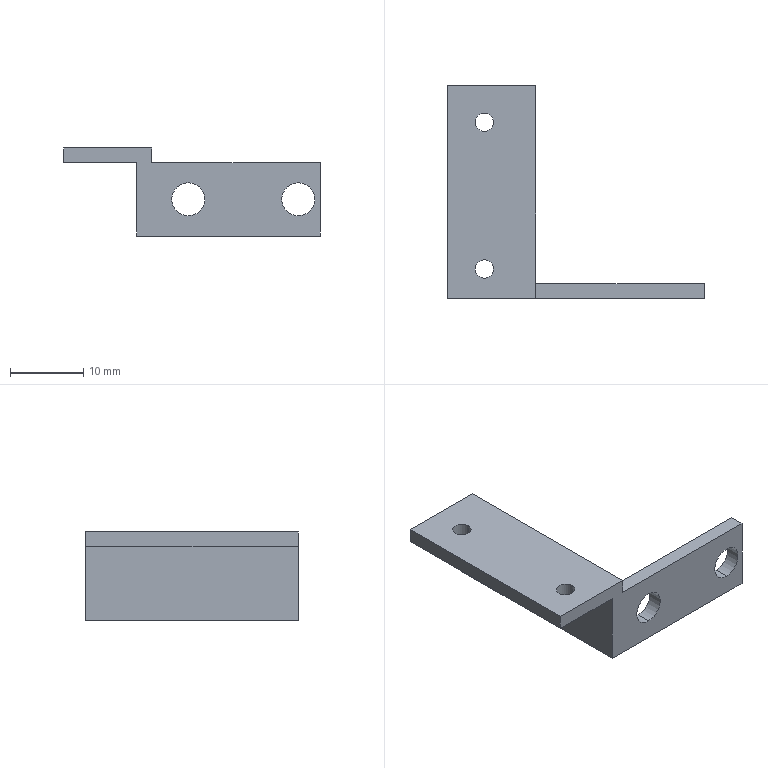Part | STEP file | switch seat | 1 solid | 19 faces | box 35 x 29 x 12 mm | volume 1653 mm3 | plane 11 | cylinder 8 | commonest cylinder face diameters 2.5 x4 4.5 x4
STEP:
#1=CARTESIAN_POINT('',(0.,0.,0.));
#2=DIRECTION('',(0.,0.,1.));
#3=DIRECTION('',(1.,0.,0.));
#4=AXIS2_PLACEMENT_3D('',#1,#2,#3);
#5=CARTESIAN_POINT('',(-5.75,8.5,10.));
#6=VERTEX_POINT('',#5);
#7=CARTESIAN_POINT('',(-5.75,8.5,12.));
#8=VERTEX_POINT('',#7);
#9=CARTESIAN_POINT('',(-5.75,8.5,12.));
#10=DIRECTION('',(0.,0.,1.));
#11=VECTOR('',#10,1.);
#12=LINE('',#9,#11);
#13=CARTESIAN_POINT('',(-7.,8.5,12.));
#14=DIRECTION('',(0.,0.,1.));
#15=DIRECTION('',(1.,0.,0.));
#16=AXIS2_PLACEMENT_3D('',#13,#14,#15);
#17=CYLINDRICAL_SURFACE('',#16,1.25);
#18=CARTESIAN_POINT('',(6.283,0.));
#19=DIRECTION('',(0.,1.));
#20=VECTOR('',#19,1.);
#21=LINE('',#18,#20);
#22=(GEOMETRIC_REPRESENTATION_CONTEXT(2)PARAMETRIC_REPRESENTATION_CONTEXT()REPRESENTATION_CONTEXT('',''));
#23=DEFINITIONAL_REPRESENTATION('',(#21),#22);
#24=PCURVE('',#17,#23);
#25=CARTESIAN_POINT('',(-7.,8.5,12.));
#26=DIRECTION('',(0.,0.,1.));
#27=DIRECTION('',(1.,0.,0.));
#28=AXIS2_PLACEMENT_3D('',#25,#26,#27);
#29=CYLINDRICAL_SURFACE('',#28,1.25);
#30=CARTESIAN_POINT('',(0.,0.));
#31=DIRECTION('',(0.,1.));
#32=VECTOR('',#31,1.);
#33=LINE('',#30,#32);
#34=(GEOMETRIC_REPRESENTATION_CONTEXT(2)PARAMETRIC_REPRESENTATION_CONTEXT()REPRESENTATION_CONTEXT('',''));
#35=DEFINITIONAL_REPRESENTATION('',(#33),#34);
#36=PCURVE('',#29,#35);
#37=SURFACE_CURVE('',#12,(#24,#36),.PCURVE_S1.);
#38=EDGE_CURVE('',#6,#8,#37,.T.);
#39=ORIENTED_EDGE('',*,*,#38,.T.);
#40=CARTESIAN_POINT('',(-8.25,8.5,12.));
#41=VERTEX_POINT('',#40);
#42=CARTESIAN_POINT('',(-7.,8.5,12.));
#43=DIRECTION('',(0.,0.,1.));
#44=DIRECTION('',(1.,0.,0.));
#45=AXIS2_PLACEMENT_3D('',#42,#43,#44);
#46=CIRCLE('',#45,1.25);
#47=CARTESIAN_POINT('',(0.,0.));
#48=DIRECTION('',(1.,0.));
#49=VECTOR('',#48,1.);
#50=LINE('',#47,#49);
#51=(GEOMETRIC_REPRESENTATION_CONTEXT(2)PARAMETRIC_REPRESENTATION_CONTEXT()REPRESENTATION_CONTEXT('',''));
#52=DEFINITIONAL_REPRESENTATION('',(#50),#51);
#53=PCURVE('',#17,#52);
#54=CARTESIAN_POINT('',(-12.,13.5,12.));
#55=DIRECTION('',(0.,0.,1.));
#56=DIRECTION('',(1.,0.,0.));
#57=AXIS2_PLACEMENT_3D('',#54,#55,#56);
#58=PLANE('',#57);
#59=CARTESIAN_POINT('',(5.,-5.));
#60=DIRECTION('',(1.,0.));
#61=AXIS2_PLACEMENT_2D('',#59,#60);
#62=CIRCLE('',#61,1.25);
#63=(GEOMETRIC_REPRESENTATION_CONTEXT(2)PARAMETRIC_REPRESENTATION_CONTEXT()REPRESENTATION_CONTEXT('',''));
#64=DEFINITIONAL_REPRESENTATION('',(#62),#63);
#65=PCURVE('',#58,#64);
#66=SURFACE_CURVE('',#46,(#53,#65),.PCURVE_S1.);
#67=EDGE_CURVE('',#41,#8,#66,.T.);
#68=ORIENTED_EDGE('',*,*,#67,.F.);
#69=CARTESIAN_POINT('',(-8.25,8.5,10.));
#70=VERTEX_POINT('',#69);
#71=CARTESIAN_POINT('',(-8.25,8.5,12.));
#72=DIRECTION('',(0.,0.,1.));
#73=VECTOR('',#72,1.);
#74=LINE('',#71,#73);
#75=CARTESIAN_POINT('',(3.142,0.));
#76=DIRECTION('',(0.,1.));
#77=VECTOR('',#76,1.);
#78=LINE('',#75,#77);
#79=(GEOMETRIC_REPRESENTATION_CONTEXT(2)PARAMETRIC_REPRESENTATION_CONTEXT()REPRESENTATION_CONTEXT('',''));
#80=DEFINITIONAL_REPRESENTATION('',(#78),#79);
#81=PCURVE('',#17,#80);
#82=CARTESIAN_POINT('',(3.142,0.));
#83=DIRECTION('',(0.,1.));
#84=VECTOR('',#83,1.);
#85=LINE('',#82,#84);
#86=(GEOMETRIC_REPRESENTATION_CONTEXT(2)PARAMETRIC_REPRESENTATION_CONTEXT()REPRESENTATION_CONTEXT('',''));
#87=DEFINITIONAL_REPRESENTATION('',(#85),#86);
#88=PCURVE('',#29,#87);
#89=SURFACE_CURVE('',#74,(#81,#88),.PCURVE_S1.);
#90=EDGE_CURVE('',#70,#41,#89,.T.);
#91=ORIENTED_EDGE('',*,*,#90,.F.);
#92=CARTESIAN_POINT('',(-7.,8.5,10.));
#93=DIRECTION('',(0.,0.,-1.));
#94=DIRECTION('',(-1.,0.,0.));
#95=AXIS2_PLACEMENT_3D('',#92,#93,#94);
#96=CIRCLE('',#95,1.25);
#97=CARTESIAN_POINT('',(9.425,-2.));
#98=DIRECTION('',(-1.,0.));
#99=VECTOR('',#98,1.);
#100=LINE('',#97,#99);
#101=(GEOMETRIC_REPRESENTATION_CONTEXT(2)PARAMETRIC_REPRESENTATION_CONTEXT()REPRESENTATION_CONTEXT('',''));
#102=DEFINITIONAL_REPRESENTATION('',(#100),#101);
#103=PCURVE('',#17,#102);
#104=CARTESIAN_POINT('',(-2.,-15.5,10.));
#105=DIRECTION('',(0.,0.,-1.));
#106=DIRECTION('',(-1.,0.,0.));
#107=AXIS2_PLACEMENT_3D('',#104,#105,#106);
#108=PLANE('',#107);
#109=CARTESIAN_POINT('',(5.,24.));
#110=DIRECTION('',(1.,0.));
#111=AXIS2_PLACEMENT_2D('',#109,#110);
#112=CIRCLE('',#111,1.25);
#113=(GEOMETRIC_REPRESENTATION_CONTEXT(2)PARAMETRIC_REPRESENTATION_CONTEXT()REPRESENTATION_CONTEXT('',''));
#114=DEFINITIONAL_REPRESENTATION('',(#112),#113);
#115=PCURVE('',#108,#114);
#116=SURFACE_CURVE('',#96,(#103,#115),.PCURVE_S1.);
#117=EDGE_CURVE('',#6,#70,#116,.T.);
#118=ORIENTED_EDGE('',*,*,#117,.F.);
#119=EDGE_LOOP('',(#39,#68,#91,#118));
#120=FACE_BOUND('',#119,.F.);
#121=ADVANCED_FACE('',(#120),#17,.F.);
#122=CARTESIAN_POINT('',(-5.75,-11.5,10.));
#123=VERTEX_POINT('',#122);
#124=CARTESIAN_POINT('',(-5.75,-11.5,12.));
#125=VERTEX_POINT('',#124);
#126=CARTESIAN_POINT('',(-5.75,-11.5,12.));
#127=DIRECTION('',(0.,0.,1.));
#128=VECTOR('',#127,1.);
#129=LINE('',#126,#128);
#130=CARTESIAN_POINT('',(-7.,-11.5,12.));
#131=DIRECTION('',(0.,0.,1.));
#132=DIRECTION('',(1.,0.,0.));
#133=AXIS2_PLACEMENT_3D('',#130,#131,#132);
#134=CYLINDRICAL_SURFACE('',#133,1.25);
#135=CARTESIAN_POINT('',(6.283,0.));
#136=DIRECTION('',(0.,1.));
#137=VECTOR('',#136,1.);
#138=LINE('',#135,#137);
#139=(GEOMETRIC_REPRESENTATION_CONTEXT(2)PARAMETRIC_REPRESENTATION_CONTEXT()REPRESENTATION_CONTEXT('',''));
#140=DEFINITIONAL_REPRESENTATION('',(#138),#139);
#141=PCURVE('',#134,#140);
#142=CARTESIAN_POINT('',(-7.,-11.5,12.));
#143=DIRECTION('',(0.,0.,1.));
#144=DIRECTION('',(1.,0.,0.));
#145=AXIS2_PLACEMENT_3D('',#142,#143,#144);
#146=CYLINDRICAL_SURFACE('',#145,1.25);
#147=CARTESIAN_POINT('',(0.,0.));
#148=DIRECTION('',(0.,1.));
#149=VECTOR('',#148,1.);
#150=LINE('',#147,#149);
#151=(GEOMETRIC_REPRESENTATION_CONTEXT(2)PARAMETRIC_REPRESENTATION_CONTEXT()REPRESENTATION_CONTEXT('',''));
#152=DEFINITIONAL_REPRESENTATION('',(#150),#151);
#153=PCURVE('',#146,#152);
#154=SURFACE_CURVE('',#129,(#141,#153),.PCURVE_S1.);
#155=EDGE_CURVE('',#123,#125,#154,.T.);
#156=ORIENTED_EDGE('',*,*,#155,.T.);
#157=CARTESIAN_POINT('',(-8.25,-11.5,12.));
#158=VERTEX_POINT('',#157);
#159=CARTESIAN_POINT('',(-7.,-11.5,12.));
#160=DIRECTION('',(0.,0.,1.));
#161=DIRECTION('',(1.,0.,0.));
#162=AXIS2_PLACEMENT_3D('',#159,#160,#161);
#163=CIRCLE('',#162,1.25);
#164=CARTESIAN_POINT('',(0.,0.));
#165=DIRECTION('',(1.,0.));
#166=VECTOR('',#165,1.);
#167=LINE('',#164,#166);
#168=(GEOMETRIC_REPRESENTATION_CONTEXT(2)PARAMETRIC_REPRESENTATION_CONTEXT()REPRESENTATION_CONTEXT('',''));
#169=DEFINITIONAL_REPRESENTATION('',(#167),#168);
#170=PCURVE('',#134,#169);
#171=CARTESIAN_POINT('',(5.,-25.));
#172=DIRECTION('',(1.,0.));
#173=AXIS2_PLACEMENT_2D('',#171,#172);
#174=CIRCLE('',#173,1.25);
#175=(GEOMETRIC_REPRESENTATION_CONTEXT(2)PARAMETRIC_REPRESENTATION_CONTEXT()REPRESENTATION_CONTEXT('',''));
#176=DEFINITIONAL_REPRESENTATION('',(#174),#175);
#177=PCURVE('',#58,#176);
#178=SURFACE_CURVE('',#163,(#170,#177),.PCURVE_S1.);
#179=EDGE_CURVE('',#158,#125,#178,.T.);
#180=ORIENTED_EDGE('',*,*,#179,.F.);
#181=CARTESIAN_POINT('',(-8.25,-11.5,10.));
#182=VERTEX_POINT('',#181);
#183=CARTESIAN_POINT('',(-8.25,-11.5,12.));
#184=DIRECTION('',(0.,0.,1.));
#185=VECTOR('',#184,1.);
#186=LINE('',#183,#185);
#187=CARTESIAN_POINT('',(3.142,0.));
#188=DIRECTION('',(0.,1.));
#189=VECTOR('',#188,1.);
#190=LINE('',#187,#189);
#191=(GEOMETRIC_REPRESENTATION_CONTEXT(2)PARAMETRIC_REPRESENTATION_CONTEXT()REPRESENTATION_CONTEXT('',''));
#192=DEFINITIONAL_REPRESENTATION('',(#190),#191);
#193=PCURVE('',#134,#192);
#194=CARTESIAN_POINT('',(3.142,0.));
#195=DIRECTION('',(0.,1.));
#196=VECTOR('',#195,1.);
#197=LINE('',#194,#196);
#198=(GEOMETRIC_REPRESENTATION_CONTEXT(2)PARAMETRIC_REPRESENTATION_CONTEXT()REPRESENTATION_CONTEXT('',''));
#199=DEFINITIONAL_REPRESENTATION('',(#197),#198);
#200=PCURVE('',#146,#199);
#201=SURFACE_CURVE('',#186,(#193,#200),.PCURVE_S1.);
#202=EDGE_CURVE('',#182,#158,#201,.T.);
#203=ORIENTED_EDGE('',*,*,#202,.F.);
#204=CARTESIAN_POINT('',(-7.,-11.5,10.));
#205=DIRECTION('',(0.,0.,-1.));
#206=DIRECTION('',(-1.,0.,0.));
#207=AXIS2_PLACEMENT_3D('',#204,#205,#206);
#208=CIRCLE('',#207,1.25);
#209=CARTESIAN_POINT('',(9.425,-2.));
#210=DIRECTION('',(-1.,0.));
#211=VECTOR('',#210,1.);
#212=LINE('',#209,#211);
#213=(GEOMETRIC_REPRESENTATION_CONTEXT(2)PARAMETRIC_REPRESENTATION_CONTEXT()REPRESENTATION_CONTEXT('',''));
#214=DEFINITIONAL_REPRESENTATION('',(#212),#213);
#215=PCURVE('',#134,#214);
#216=CARTESIAN_POINT('',(5.,4.));
#217=DIRECTION('',(1.,0.));
#218=AXIS2_PLACEMENT_2D('',#216,#217);
#219=CIRCLE('',#218,1.25);
#220=(GEOMETRIC_REPRESENTATION_CONTEXT(2)PARAMETRIC_REPRESENTATION_CONTEXT()REPRESENTATION_CONTEXT('',''));
#221=DEFINITIONAL_REPRESENTATION('',(#219),#220);
#222=PCURVE('',#108,#221);
#223=SURFACE_CURVE('',#208,(#215,#222),.PCURVE_S1.);
#224=EDGE_CURVE('',#123,#182,#223,.T.);
#225=ORIENTED_EDGE('',*,*,#224,.F.);
#226=EDGE_LOOP('',(#156,#180,#203,#225));
#227=FACE_BOUND('',#226,.F.);
#228=ADVANCED_FACE('',(#227),#134,.F.);
#229=CARTESIAN_POINT('',(4.993,-15.5,7.25));
#230=VERTEX_POINT('',#229);
#231=CARTESIAN_POINT('',(4.993,-13.5,7.25));
#232=VERTEX_POINT('',#231);
#233=CARTESIAN_POINT('',(4.993,-15.5,7.25));
#234=DIRECTION('',(0.,1.,0.));
#235=VECTOR('',#234,1.);
#236=LINE('',#233,#235);
#237=CARTESIAN_POINT('',(4.993,-15.5,5.));
#238=DIRECTION('',(0.,1.,0.));
#239=DIRECTION('',(0.,0.,1.));
#240=AXIS2_PLACEMENT_3D('',#237,#238,#239);
#241=CYLINDRICAL_SURFACE('',#240,2.25);
#242=CARTESIAN_POINT('',(6.283,0.));
#243=DIRECTION('',(0.,1.));
#244=VECTOR('',#243,1.);
#245=LINE('',#242,#244);
#246=(GEOMETRIC_REPRESENTATION_CONTEXT(2)PARAMETRIC_REPRESENTATION_CONTEXT()REPRESENTATION_CONTEXT('',''));
#247=DEFINITIONAL_REPRESENTATION('',(#245),#246);
#248=PCURVE('',#241,#247);
#249=CARTESIAN_POINT('',(4.993,-15.5,5.));
#250=DIRECTION('',(0.,1.,0.));
#251=DIRECTION('',(0.,0.,1.));
#252=AXIS2_PLACEMENT_3D('',#249,#250,#251);
#253=CYLINDRICAL_SURFACE('',#252,2.25);
#254=CARTESIAN_POINT('',(0.,0.));
#255=DIRECTION('',(0.,1.));
#256=VECTOR('',#255,1.);
#257=LINE('',#254,#256);
#258=(GEOMETRIC_REPRESENTATION_CONTEXT(2)PARAMETRIC_REPRESENTATION_CONTEXT()REPRESENTATION_CONTEXT('',''));
#259=DEFINITIONAL_REPRESENTATION('',(#257),#258);
#260=PCURVE('',#253,#259);
#261=SURFACE_CURVE('',#236,(#248,#260),.PCURVE_S1.);
#262=EDGE_CURVE('',#230,#232,#261,.T.);
#263=ORIENTED_EDGE('',*,*,#262,.T.);
#264=CARTESIAN_POINT('',(4.993,-13.5,2.75));
#265=VERTEX_POINT('',#264);
#266=CARTESIAN_POINT('',(4.993,-13.5,5.));
#267=DIRECTION('',(0.,-1.,0.));
#268=DIRECTION('',(0.,0.,-1.));
#269=AXIS2_PLACEMENT_3D('',#266,#267,#268);
#270=CIRCLE('',#269,2.25);
#271=CARTESIAN_POINT('',(9.425,2.));
#272=DIRECTION('',(-1.,0.));
#273=VECTOR('',#272,1.);
#274=LINE('',#271,#273);
#275=(GEOMETRIC_REPRESENTATION_CONTEXT(2)PARAMETRIC_REPRESENTATION_CONTEXT()REPRESENTATION_CONTEXT('',''));
#276=DEFINITIONAL_REPRESENTATION('',(#274),#275);
#277=PCURVE('',#241,#276);
#278=CARTESIAN_POINT('',(23.,-13.5,12.));
#279=DIRECTION('',(0.,-1.,0.));
#280=DIRECTION('',(0.,0.,-1.));
#281=AXIS2_PLACEMENT_3D('',#278,#279,#280);
#282=PLANE('',#281);
#283=CARTESIAN_POINT('',(7.,-18.007));
#284=DIRECTION('',(1.,0.));
#285=AXIS2_PLACEMENT_2D('',#283,#284);
#286=CIRCLE('',#285,2.25);
#287=(GEOMETRIC_REPRESENTATION_CONTEXT(2)PARAMETRIC_REPRESENTATION_CONTEXT()REPRESENTATION_CONTEXT('',''));
#288=DEFINITIONAL_REPRESENTATION('',(#286),#287);
#289=PCURVE('',#282,#288);
#290=SURFACE_CURVE('',#270,(#277,#289),.PCURVE_S1.);
#291=EDGE_CURVE('',#232,#265,#290,.T.);
#292=ORIENTED_EDGE('',*,*,#291,.T.);
#293=CARTESIAN_POINT('',(4.993,-15.5,2.75));
#294=VERTEX_POINT('',#293);
#295=CARTESIAN_POINT('',(4.993,-15.5,2.75));
#296=DIRECTION('',(0.,1.,0.));
#297=VECTOR('',#296,1.);
#298=LINE('',#295,#297);
#299=CARTESIAN_POINT('',(3.142,0.));
#300=DIRECTION('',(0.,1.));
#301=VECTOR('',#300,1.);
#302=LINE('',#299,#301);
#303=(GEOMETRIC_REPRESENTATION_CONTEXT(2)PARAMETRIC_REPRESENTATION_CONTEXT()REPRESENTATION_CONTEXT('',''));
#304=DEFINITIONAL_REPRESENTATION('',(#302),#303);
#305=PCURVE('',#241,#304);
#306=CARTESIAN_POINT('',(3.142,0.));
#307=DIRECTION('',(0.,1.));
#308=VECTOR('',#307,1.);
#309=LINE('',#306,#308);
#310=(GEOMETRIC_REPRESENTATION_CONTEXT(2)PARAMETRIC_REPRESENTATION_CONTEXT()REPRESENTATION_CONTEXT('',''));
#311=DEFINITIONAL_REPRESENTATION('',(#309),#310);
#312=PCURVE('',#253,#311);
#313=SURFACE_CURVE('',#298,(#305,#312),.PCURVE_S1.);
#314=EDGE_CURVE('',#294,#265,#313,.T.);
#315=ORIENTED_EDGE('',*,*,#314,.F.);
#316=CARTESIAN_POINT('',(4.993,-15.5,5.));
#317=DIRECTION('',(0.,1.,0.));
#318=DIRECTION('',(0.,0.,1.));
#319=AXIS2_PLACEMENT_3D('',#316,#317,#318);
#320=CIRCLE('',#319,2.25);
#321=CARTESIAN_POINT('',(0.,0.));
#322=DIRECTION('',(1.,0.));
#323=VECTOR('',#322,1.);
#324=LINE('',#321,#323);
#325=(GEOMETRIC_REPRESENTATION_CONTEXT(2)PARAMETRIC_REPRESENTATION_CONTEXT()REPRESENTATION_CONTEXT('',''));
#326=DEFINITIONAL_REPRESENTATION('',(#324),#325);
#327=PCURVE('',#241,#326);
#328=CARTESIAN_POINT('',(23.,-15.5,12.));
#329=DIRECTION('',(0.,1.,0.));
#330=DIRECTION('',(0.,0.,1.));
#331=AXIS2_PLACEMENT_3D('',#328,#329,#330);
#332=PLANE('',#331);
#333=CARTESIAN_POINT('',(-7.,-18.007));
#334=DIRECTION('',(1.,0.));
#335=AXIS2_PLACEMENT_2D('',#333,#334);
#336=CIRCLE('',#335,2.25);
#337=(GEOMETRIC_REPRESENTATION_CONTEXT(2)PARAMETRIC_REPRESENTATION_CONTEXT()REPRESENTATION_CONTEXT('',''));
#338=DEFINITIONAL_REPRESENTATION('',(#336),#337);
#339=PCURVE('',#332,#338);
#340=SURFACE_CURVE('',#320,(#327,#339),.PCURVE_S1.);
#341=EDGE_CURVE('',#294,#230,#340,.T.);
#342=ORIENTED_EDGE('',*,*,#341,.T.);
#343=EDGE_LOOP('',(#263,#292,#315,#342));
#344=FACE_BOUND('',#343,.F.);
#345=ADVANCED_FACE('',(#344),#241,.F.);
#346=CARTESIAN_POINT('',(19.993,-15.5,7.25));
#347=VERTEX_POINT('',#346);
#348=CARTESIAN_POINT('',(19.993,-13.5,7.25));
#349=VERTEX_POINT('',#348);
#350=CARTESIAN_POINT('',(19.993,-15.5,7.25));
#351=DIRECTION('',(0.,1.,0.));
#352=VECTOR('',#351,1.);
#353=LINE('',#350,#352);
#354=CARTESIAN_POINT('',(19.993,-15.5,5.));
#355=DIRECTION('',(0.,1.,0.));
#356=DIRECTION('',(0.,0.,1.));
#357=AXIS2_PLACEMENT_3D('',#354,#355,#356);
#358=CYLINDRICAL_SURFACE('',#357,2.25);
#359=CARTESIAN_POINT('',(6.283,0.));
#360=DIRECTION('',(0.,1.));
#361=VECTOR('',#360,1.);
#362=LINE('',#359,#361);
#363=(GEOMETRIC_REPRESENTATION_CONTEXT(2)PARAMETRIC_REPRESENTATION_CONTEXT()REPRESENTATION_CONTEXT('',''));
#364=DEFINITIONAL_REPRESENTATION('',(#362),#363);
#365=PCURVE('',#358,#364);
#366=CARTESIAN_POINT('',(19.993,-15.5,5.));
#367=DIRECTION('',(0.,1.,0.));
#368=DIRECTION('',(0.,0.,1.));
#369=AXIS2_PLACEMENT_3D('',#366,#367,#368);
#370=CYLINDRICAL_SURFACE('',#369,2.25);
#371=CARTESIAN_POINT('',(0.,0.));
#372=DIRECTION('',(0.,1.));
#373=VECTOR('',#372,1.);
#374=LINE('',#371,#373);
#375=(GEOMETRIC_REPRESENTATION_CONTEXT(2)PARAMETRIC_REPRESENTATION_CONTEXT()REPRESENTATION_CONTEXT('',''));
#376=DEFINITIONAL_REPRESENTATION('',(#374),#375);
#377=PCURVE('',#370,#376);
#378=SURFACE_CURVE('',#353,(#365,#377),.PCURVE_S1.);
#379=EDGE_CURVE('',#347,#349,#378,.T.);
#380=ORIENTED_EDGE('',*,*,#379,.T.);
#381=CARTESIAN_POINT('',(19.993,-13.5,2.75));
#382=VERTEX_POINT('',#381);
#383=CARTESIAN_POINT('',(19.993,-13.5,5.));
#384=DIRECTION('',(0.,-1.,0.));
#385=DIRECTION('',(0.,0.,-1.));
#386=AXIS2_PLACEMENT_3D('',#383,#384,#385);
#387=CIRCLE('',#386,2.25);
#388=CARTESIAN_POINT('',(9.425,2.));
#389=DIRECTION('',(-1.,0.));
#390=VECTOR('',#389,1.);
#391=LINE('',#388,#390);
#392=(GEOMETRIC_REPRESENTATION_CONTEXT(2)PARAMETRIC_REPRESENTATION_CONTEXT()REPRESENTATION_CONTEXT('',''));
#393=DEFINITIONAL_REPRESENTATION('',(#391),#392);
#394=PCURVE('',#358,#393);
#395=CARTESIAN_POINT('',(7.,-3.007));
#396=DIRECTION('',(1.,0.));
#397=AXIS2_PLACEMENT_2D('',#395,#396);
#398=CIRCLE('',#397,2.25);
#399=(GEOMETRIC_REPRESENTATION_CONTEXT(2)PARAMETRIC_REPRESENTATION_CONTEXT()REPRESENTATION_CONTEXT('',''));
#400=DEFINITIONAL_REPRESENTATION('',(#398),#399);
#401=PCURVE('',#282,#400);
#402=SURFACE_CURVE('',#387,(#394,#401),.PCURVE_S1.);
#403=EDGE_CURVE('',#349,#382,#402,.T.);
#404=ORIENTED_EDGE('',*,*,#403,.T.);
#405=CARTESIAN_POINT('',(19.993,-15.5,2.75));
#406=VERTEX_POINT('',#405);
#407=CARTESIAN_POINT('',(19.993,-15.5,2.75));
#408=DIRECTION('',(0.,1.,0.));
#409=VECTOR('',#408,1.);
#410=LINE('',#407,#409);
#411=CARTESIAN_POINT('',(3.142,0.));
#412=DIRECTION('',(0.,1.));
#413=VECTOR('',#412,1.);
#414=LINE('',#411,#413);
#415=(GEOMETRIC_REPRESENTATION_CONTEXT(2)PARAMETRIC_REPRESENTATION_CONTEXT()REPRESENTATION_CONTEXT('',''));
#416=DEFINITIONAL_REPRESENTATION('',(#414),#415);
#417=PCURVE('',#358,#416);
#418=CARTESIAN_POINT('',(3.142,0.));
#419=DIRECTION('',(0.,1.));
#420=VECTOR('',#419,1.);
#421=LINE('',#418,#420);
#422=(GEOMETRIC_REPRESENTATION_CONTEXT(2)PARAMETRIC_REPRESENTATION_CONTEXT()REPRESENTATION_CONTEXT('',''));
#423=DEFINITIONAL_REPRESENTATION('',(#421),#422);
#424=PCURVE('',#370,#423);
#425=SURFACE_CURVE('',#410,(#417,#424),.PCURVE_S1.);
#426=EDGE_CURVE('',#406,#382,#425,.T.);
#427=ORIENTED_EDGE('',*,*,#426,.F.);
#428=CARTESIAN_POINT('',(19.993,-15.5,5.));
#429=DIRECTION('',(0.,1.,0.));
#430=DIRECTION('',(0.,0.,1.));
#431=AXIS2_PLACEMENT_3D('',#428,#429,#430);
#432=CIRCLE('',#431,2.25);
#433=CARTESIAN_POINT('',(0.,0.));
#434=DIRECTION('',(1.,0.));
#435=VECTOR('',#434,1.);
#436=LINE('',#433,#435);
#437=(GEOMETRIC_REPRESENTATION_CONTEXT(2)PARAMETRIC_REPRESENTATION_CONTEXT()REPRESENTATION_CONTEXT('',''));
#438=DEFINITIONAL_REPRESENTATION('',(#436),#437);
#439=PCURVE('',#358,#438);
#440=CARTESIAN_POINT('',(-7.,-3.007));
#441=DIRECTION('',(1.,0.));
#442=AXIS2_PLACEMENT_2D('',#440,#441);
#443=CIRCLE('',#442,2.25);
#444=(GEOMETRIC_REPRESENTATION_CONTEXT(2)PARAMETRIC_REPRESENTATION_CONTEXT()REPRESENTATION_CONTEXT('',''));
#445=DEFINITIONAL_REPRESENTATION('',(#443),#444);
#446=PCURVE('',#332,#445);
#447=SURFACE_CURVE('',#432,(#439,#446),.PCURVE_S1.);
#448=EDGE_CURVE('',#406,#347,#447,.T.);
#449=ORIENTED_EDGE('',*,*,#448,.T.);
#450=EDGE_LOOP('',(#380,#404,#427,#449));
#451=FACE_BOUND('',#450,.F.);
#452=ADVANCED_FACE('',(#451),#358,.F.);
#453=CARTESIAN_POINT('',(-7.,8.5,12.));
#454=DIRECTION('',(0.,0.,1.));
#455=DIRECTION('',(1.,0.,0.));
#456=AXIS2_PLACEMENT_3D('',#453,#454,#455);
#457=CIRCLE('',#456,1.25);
#458=CARTESIAN_POINT('',(5.,-5.));
#459=DIRECTION('',(1.,0.));
#460=AXIS2_PLACEMENT_2D('',#458,#459);
#461=CIRCLE('',#460,1.25);
#462=(GEOMETRIC_REPRESENTATION_CONTEXT(2)PARAMETRIC_REPRESENTATION_CONTEXT()REPRESENTATION_CONTEXT('',''));
#463=DEFINITIONAL_REPRESENTATION('',(#461),#462);
#464=PCURVE('',#58,#463);
#465=CARTESIAN_POINT('',(0.,0.));
#466=DIRECTION('',(1.,0.));
#467=VECTOR('',#466,1.);
#468=LINE('',#465,#467);
#469=(GEOMETRIC_REPRESENTATION_CONTEXT(2)PARAMETRIC_REPRESENTATION_CONTEXT()REPRESENTATION_CONTEXT('',''));
#470=DEFINITIONAL_REPRESENTATION('',(#468),#469);
#471=PCURVE('',#29,#470);
#472=SURFACE_CURVE('',#457,(#464,#471),.PCURVE_S1.);
#473=EDGE_CURVE('',#8,#41,#472,.T.);
#474=ORIENTED_EDGE('',*,*,#473,.F.);
#475=ORIENTED_EDGE('',*,*,#67,.F.);
#476=EDGE_LOOP('',(#474,#475));
#477=FACE_BOUND('',#476,.T.);
#478=CARTESIAN_POINT('',(-7.,-11.5,12.));
#479=DIRECTION('',(0.,0.,1.));
#480=DIRECTION('',(1.,0.,0.));
#481=AXIS2_PLACEMENT_3D('',#478,#479,#480);
#482=CIRCLE('',#481,1.25);
#483=CARTESIAN_POINT('',(5.,-25.));
#484=DIRECTION('',(1.,0.));
#485=AXIS2_PLACEMENT_2D('',#483,#484);
#486=CIRCLE('',#485,1.25);
#487=(GEOMETRIC_REPRESENTATION_CONTEXT(2)PARAMETRIC_REPRESENTATION_CONTEXT()REPRESENTATION_CONTEXT('',''));
#488=DEFINITIONAL_REPRESENTATION('',(#486),#487);
#489=PCURVE('',#58,#488);
#490=CARTESIAN_POINT('',(0.,0.));
#491=DIRECTION('',(1.,0.));
#492=VECTOR('',#491,1.);
#493=LINE('',#490,#492);
#494=(GEOMETRIC_REPRESENTATION_CONTEXT(2)PARAMETRIC_REPRESENTATION_CONTEXT()REPRESENTATION_CONTEXT('',''));
#495=DEFINITIONAL_REPRESENTATION('',(#493),#494);
#496=PCURVE('',#146,#495);
#497=SURFACE_CURVE('',#482,(#489,#496),.PCURVE_S1.);
#498=EDGE_CURVE('',#125,#158,#497,.T.);
#499=ORIENTED_EDGE('',*,*,#498,.F.);
#500=ORIENTED_EDGE('',*,*,#179,.F.);
#501=EDGE_LOOP('',(#499,#500));
#502=FACE_BOUND('',#501,.T.);
#503=CARTESIAN_POINT('',(-12.,-15.5,12.));
#504=VERTEX_POINT('',#503);
#505=CARTESIAN_POINT('',(0.,-15.5,12.));
#506=VERTEX_POINT('',#505);
#507=CARTESIAN_POINT('',(23.,-15.5,12.));
#508=DIRECTION('',(1.,0.,0.));
#509=VECTOR('',#508,1.);
#510=LINE('',#507,#509);
#511=CARTESIAN_POINT('',(35.,-29.));
#512=DIRECTION('',(1.,0.));
#513=VECTOR('',#512,1.);
#514=LINE('',#511,#513);
#515=(GEOMETRIC_REPRESENTATION_CONTEXT(2)PARAMETRIC_REPRESENTATION_CONTEXT()REPRESENTATION_CONTEXT('',''));
#516=DEFINITIONAL_REPRESENTATION('',(#514),#515);
#517=PCURVE('',#58,#516);
#518=CARTESIAN_POINT('',(0.,0.));
#519=DIRECTION('',(0.,1.));
#520=VECTOR('',#519,1.);
#521=LINE('',#518,#520);
#522=(GEOMETRIC_REPRESENTATION_CONTEXT(2)PARAMETRIC_REPRESENTATION_CONTEXT()REPRESENTATION_CONTEXT('',''));
#523=DEFINITIONAL_REPRESENTATION('',(#521),#522);
#524=PCURVE('',#332,#523);
#525=SURFACE_CURVE('',#510,(#517,#524),.PCURVE_S1.);
#526=EDGE_CURVE('',#504,#506,#525,.T.);
#527=ORIENTED_EDGE('',*,*,#526,.T.);
#528=CARTESIAN_POINT('',(0.,13.5,12.));
#529=VERTEX_POINT('',#528);
#530=CARTESIAN_POINT('',(0.,-13.5,12.));
#531=DIRECTION('',(0.,1.,0.));
#532=VECTOR('',#531,1.);
#533=LINE('',#530,#532);
#534=CARTESIAN_POINT('',(12.,-27.));
#535=DIRECTION('',(0.,1.));
#536=VECTOR('',#535,1.);
#537=LINE('',#534,#536);
#538=(GEOMETRIC_REPRESENTATION_CONTEXT(2)PARAMETRIC_REPRESENTATION_CONTEXT()REPRESENTATION_CONTEXT('',''));
#539=DEFINITIONAL_REPRESENTATION('',(#537),#538);
#540=PCURVE('',#58,#539);
#541=CARTESIAN_POINT('',(0.,-13.5,12.));
#542=DIRECTION('',(-1.,0.,0.));
#543=DIRECTION('',(0.,0.,1.));
#544=AXIS2_PLACEMENT_3D('',#541,#542,#543);
#545=PLANE('',#544);
#546=CARTESIAN_POINT('',(0.,0.));
#547=DIRECTION('',(0.,1.));
#548=VECTOR('',#547,1.);
#549=LINE('',#546,#548);
#550=(GEOMETRIC_REPRESENTATION_CONTEXT(2)PARAMETRIC_REPRESENTATION_CONTEXT()REPRESENTATION_CONTEXT('',''));
#551=DEFINITIONAL_REPRESENTATION('',(#549),#550);
#552=PCURVE('',#545,#551);
#553=SURFACE_CURVE('',#533,(#540,#552),.PCURVE_S1.);
#554=EDGE_CURVE('',#506,#529,#553,.T.);
#555=ORIENTED_EDGE('',*,*,#554,.T.);
#556=CARTESIAN_POINT('',(-12.,13.5,12.));
#557=VERTEX_POINT('',#556);
#558=CARTESIAN_POINT('',(0.,13.5,12.));
#559=DIRECTION('',(-1.,0.,0.));
#560=VECTOR('',#559,1.);
#561=LINE('',#558,#560);
#562=CARTESIAN_POINT('',(12.,0.));
#563=DIRECTION('',(-1.,0.));
#564=VECTOR('',#563,1.);
#565=LINE('',#562,#564);
#566=(GEOMETRIC_REPRESENTATION_CONTEXT(2)PARAMETRIC_REPRESENTATION_CONTEXT()REPRESENTATION_CONTEXT('',''));
#567=DEFINITIONAL_REPRESENTATION('',(#565),#566);
#568=PCURVE('',#58,#567);
#569=CARTESIAN_POINT('',(0.,13.5,12.));
#570=DIRECTION('',(0.,-1.,0.));
#571=DIRECTION('',(0.,0.,-1.));
#572=AXIS2_PLACEMENT_3D('',#569,#570,#571);
#573=PLANE('',#572);
#574=CARTESIAN_POINT('',(0.,0.));
#575=DIRECTION('',(0.,-1.));
#576=VECTOR('',#575,1.);
#577=LINE('',#574,#576);
#578=(GEOMETRIC_REPRESENTATION_CONTEXT(2)PARAMETRIC_REPRESENTATION_CONTEXT()REPRESENTATION_CONTEXT('',''));
#579=DEFINITIONAL_REPRESENTATION('',(#577),#578);
#580=PCURVE('',#573,#579);
#581=SURFACE_CURVE('',#561,(#568,#580),.PCURVE_S1.);
#582=EDGE_CURVE('',#529,#557,#581,.T.);
#583=ORIENTED_EDGE('',*,*,#582,.T.);
#584=CARTESIAN_POINT('',(-12.,13.5,12.));
#585=DIRECTION('',(0.,-1.,0.));
#586=VECTOR('',#585,1.);
#587=LINE('',#584,#586);
#588=CARTESIAN_POINT('',(0.,0.));
#589=DIRECTION('',(0.,-1.));
#590=VECTOR('',#589,1.);
#591=LINE('',#588,#590);
#592=(GEOMETRIC_REPRESENTATION_CONTEXT(2)PARAMETRIC_REPRESENTATION_CONTEXT()REPRESENTATION_CONTEXT('',''));
#593=DEFINITIONAL_REPRESENTATION('',(#591),#592);
#594=PCURVE('',#58,#593);
#595=CARTESIAN_POINT('',(-12.,13.5,12.));
#596=DIRECTION('',(1.,0.,0.));
#597=DIRECTION('',(0.,0.,-1.));
#598=AXIS2_PLACEMENT_3D('',#595,#596,#597);
#599=PLANE('',#598);
#600=CARTESIAN_POINT('',(0.,0.));
#601=DIRECTION('',(0.,-1.));
#602=VECTOR('',#601,1.);
#603=LINE('',#600,#602);
#604=(GEOMETRIC_REPRESENTATION_CONTEXT(2)PARAMETRIC_REPRESENTATION_CONTEXT()REPRESENTATION_CONTEXT('',''));
#605=DEFINITIONAL_REPRESENTATION('',(#603),#604);
#606=PCURVE('',#599,#605);
#607=SURFACE_CURVE('',#587,(#594,#606),.PCURVE_S1.);
#608=EDGE_CURVE('',#557,#504,#607,.T.);
#609=ORIENTED_EDGE('',*,*,#608,.T.);
#610=EDGE_LOOP('',(#527,#555,#583,#609));
#611=FACE_BOUND('',#610,.T.);
#612=ADVANCED_FACE('',(#477,#502,#611),#58,.T.);
#613=CARTESIAN_POINT('',(-2.,-15.5,0.));
#614=VERTEX_POINT('',#613);
#615=CARTESIAN_POINT('',(-2.,13.5,0.));
#616=VERTEX_POINT('',#615);
#617=CARTESIAN_POINT('',(-2.,-15.5,0.));
#618=DIRECTION('',(0.,1.,0.));
#619=VECTOR('',#618,1.);
#620=LINE('',#617,#619);
#621=CARTESIAN_POINT('',(-12.,13.5,0.));
#622=DIRECTION('',(0.,0.,1.));
#623=DIRECTION('',(1.,0.,0.));
#624=AXIS2_PLACEMENT_3D('',#621,#622,#623);
#625=PLANE('',#624);
#626=CARTESIAN_POINT('',(10.,-29.));
#627=DIRECTION('',(0.,1.));
#628=VECTOR('',#627,1.);
#629=LINE('',#626,#628);
#630=(GEOMETRIC_REPRESENTATION_CONTEXT(2)PARAMETRIC_REPRESENTATION_CONTEXT()REPRESENTATION_CONTEXT('',''));
#631=DEFINITIONAL_REPRESENTATION('',(#629),#630);
#632=PCURVE('',#625,#631);
#633=CARTESIAN_POINT('',(-2.,-15.5,0.));
#634=DIRECTION('',(-1.,0.,0.));
#635=DIRECTION('',(0.,0.,1.));
#636=AXIS2_PLACEMENT_3D('',#633,#634,#635);
#637=PLANE('',#636);
#638=CARTESIAN_POINT('',(0.,0.));
#639=DIRECTION('',(0.,1.));
#640=VECTOR('',#639,1.);
#641=LINE('',#638,#640);
#642=(GEOMETRIC_REPRESENTATION_CONTEXT(2)PARAMETRIC_REPRESENTATION_CONTEXT()REPRESENTATION_CONTEXT('',''));
#643=DEFINITIONAL_REPRESENTATION('',(#641),#642);
#644=PCURVE('',#637,#643);
#645=SURFACE_CURVE('',#620,(#632,#644),.PCURVE_S1.);
#646=EDGE_CURVE('',#614,#616,#645,.T.);
#647=ORIENTED_EDGE('',*,*,#646,.T.);
#648=CARTESIAN_POINT('',(0.,13.5,0.));
#649=VERTEX_POINT('',#648);
#650=CARTESIAN_POINT('',(0.,13.5,0.));
#651=DIRECTION('',(-1.,0.,0.));
#652=VECTOR('',#651,1.);
#653=LINE('',#650,#652);
#654=CARTESIAN_POINT('',(12.,0.));
#655=DIRECTION('',(-1.,0.));
#656=VECTOR('',#655,1.);
#657=LINE('',#654,#656);
#658=(GEOMETRIC_REPRESENTATION_CONTEXT(2)PARAMETRIC_REPRESENTATION_CONTEXT()REPRESENTATION_CONTEXT('',''));
#659=DEFINITIONAL_REPRESENTATION('',(#657),#658);
#660=PCURVE('',#625,#659);
#661=CARTESIAN_POINT('',(12.,0.));
#662=DIRECTION('',(0.,-1.));
#663=VECTOR('',#662,1.);
#664=LINE('',#661,#663);
#665=(GEOMETRIC_REPRESENTATION_CONTEXT(2)PARAMETRIC_REPRESENTATION_CONTEXT()REPRESENTATION_CONTEXT('',''));
#666=DEFINITIONAL_REPRESENTATION('',(#664),#665);
#667=PCURVE('',#573,#666);
#668=SURFACE_CURVE('',#653,(#660,#667),.PCURVE_S1.);
#669=EDGE_CURVE('',#649,#616,#668,.T.);
#670=ORIENTED_EDGE('',*,*,#669,.F.);
#671=CARTESIAN_POINT('',(0.,-13.5,0.));
#672=VERTEX_POINT('',#671);
#673=CARTESIAN_POINT('',(0.,-13.5,0.));
#674=DIRECTION('',(0.,1.,0.));
#675=VECTOR('',#674,1.);
#676=LINE('',#673,#675);
#677=CARTESIAN_POINT('',(12.,-27.));
#678=DIRECTION('',(0.,1.));
#679=VECTOR('',#678,1.);
#680=LINE('',#677,#679);
#681=(GEOMETRIC_REPRESENTATION_CONTEXT(2)PARAMETRIC_REPRESENTATION_CONTEXT()REPRESENTATION_CONTEXT('',''));
#682=DEFINITIONAL_REPRESENTATION('',(#680),#681);
#683=PCURVE('',#625,#682);
#684=CARTESIAN_POINT('',(-12.,0.));
#685=DIRECTION('',(0.,1.));
#686=VECTOR('',#685,1.);
#687=LINE('',#684,#686);
#688=(GEOMETRIC_REPRESENTATION_CONTEXT(2)PARAMETRIC_REPRESENTATION_CONTEXT()REPRESENTATION_CONTEXT('',''));
#689=DEFINITIONAL_REPRESENTATION('',(#687),#688);
#690=PCURVE('',#545,#689);
#691=SURFACE_CURVE('',#676,(#683,#690),.PCURVE_S1.);
#692=EDGE_CURVE('',#672,#649,#691,.T.);
#693=ORIENTED_EDGE('',*,*,#692,.F.);
#694=CARTESIAN_POINT('',(23.,-13.5,0.));
#695=VERTEX_POINT('',#694);
#696=CARTESIAN_POINT('',(23.,-13.5,0.));
#697=DIRECTION('',(-1.,0.,0.));
#698=VECTOR('',#697,1.);
#699=LINE('',#696,#698);
#700=CARTESIAN_POINT('',(35.,-27.));
#701=DIRECTION('',(-1.,0.));
#702=VECTOR('',#701,1.);
#703=LINE('',#700,#702);
#704=(GEOMETRIC_REPRESENTATION_CONTEXT(2)PARAMETRIC_REPRESENTATION_CONTEXT()REPRESENTATION_CONTEXT('',''));
#705=DEFINITIONAL_REPRESENTATION('',(#703),#704);
#706=PCURVE('',#625,#705);
#707=CARTESIAN_POINT('',(12.,0.));
#708=DIRECTION('',(0.,-1.));
#709=VECTOR('',#708,1.);
#710=LINE('',#707,#709);
#711=(GEOMETRIC_REPRESENTATION_CONTEXT(2)PARAMETRIC_REPRESENTATION_CONTEXT()REPRESENTATION_CONTEXT('',''));
#712=DEFINITIONAL_REPRESENTATION('',(#710),#711);
#713=PCURVE('',#282,#712);
#714=SURFACE_CURVE('',#699,(#706,#713),.PCURVE_S1.);
#715=EDGE_CURVE('',#695,#672,#714,.T.);
#716=ORIENTED_EDGE('',*,*,#715,.F.);
#717=CARTESIAN_POINT('',(23.,-15.5,0.));
#718=VERTEX_POINT('',#717);
#719=CARTESIAN_POINT('',(23.,-13.5,0.));
#720=DIRECTION('',(0.,1.,0.));
#721=VECTOR('',#720,1.);
#722=LINE('',#719,#721);
#723=CARTESIAN_POINT('',(35.,-27.));
#724=DIRECTION('',(0.,1.));
#725=VECTOR('',#724,1.);
#726=LINE('',#723,#725);
#727=(GEOMETRIC_REPRESENTATION_CONTEXT(2)PARAMETRIC_REPRESENTATION_CONTEXT()REPRESENTATION_CONTEXT('',''));
#728=DEFINITIONAL_REPRESENTATION('',(#726),#727);
#729=PCURVE('',#625,#728);
#730=CARTESIAN_POINT('',(23.,-13.5,12.));
#731=DIRECTION('',(-1.,0.,0.));
#732=DIRECTION('',(0.,0.,1.));
#733=AXIS2_PLACEMENT_3D('',#730,#731,#732);
#734=PLANE('',#733);
#735=CARTESIAN_POINT('',(-12.,0.));
#736=DIRECTION('',(0.,1.));
#737=VECTOR('',#736,1.);
#738=LINE('',#735,#737);
#739=(GEOMETRIC_REPRESENTATION_CONTEXT(2)PARAMETRIC_REPRESENTATION_CONTEXT()REPRESENTATION_CONTEXT('',''));
#740=DEFINITIONAL_REPRESENTATION('',(#738),#739);
#741=PCURVE('',#734,#740);
#742=SURFACE_CURVE('',#722,(#729,#741),.PCURVE_S1.);
#743=EDGE_CURVE('',#718,#695,#742,.T.);
#744=ORIENTED_EDGE('',*,*,#743,.F.);
#745=CARTESIAN_POINT('',(23.,-15.5,0.));
#746=DIRECTION('',(1.,0.,0.));
#747=VECTOR('',#746,1.);
#748=LINE('',#745,#747);
#749=CARTESIAN_POINT('',(35.,-29.));
#750=DIRECTION('',(1.,0.));
#751=VECTOR('',#750,1.);
#752=LINE('',#749,#751);
#753=(GEOMETRIC_REPRESENTATION_CONTEXT(2)PARAMETRIC_REPRESENTATION_CONTEXT()REPRESENTATION_CONTEXT('',''));
#754=DEFINITIONAL_REPRESENTATION('',(#752),#753);
#755=PCURVE('',#625,#754);
#756=CARTESIAN_POINT('',(-12.,0.));
#757=DIRECTION('',(0.,1.));
#758=VECTOR('',#757,1.);
#759=LINE('',#756,#758);
#760=(GEOMETRIC_REPRESENTATION_CONTEXT(2)PARAMETRIC_REPRESENTATION_CONTEXT()REPRESENTATION_CONTEXT('',''));
#761=DEFINITIONAL_REPRESENTATION('',(#759),#760);
#762=PCURVE('',#332,#761);
#763=SURFACE_CURVE('',#748,(#755,#762),.PCURVE_S1.);
#764=EDGE_CURVE('',#614,#718,#763,.T.);
#765=ORIENTED_EDGE('',*,*,#764,.F.);
#766=EDGE_LOOP('',(#647,#670,#693,#716,#744,#765));
#767=FACE_BOUND('',#766,.T.);
#768=ADVANCED_FACE('',(#767),#625,.F.);
#769=CARTESIAN_POINT('',(-2.,13.5,10.));
#770=VERTEX_POINT('',#769);
#771=CARTESIAN_POINT('',(-2.,13.5,0.));
#772=DIRECTION('',(0.,0.,1.));
#773=VECTOR('',#772,1.);
#774=LINE('',#771,#773);
#775=CARTESIAN_POINT('',(12.,-2.));
#776=DIRECTION('',(-1.,0.));
#777=VECTOR('',#776,1.);
#778=LINE('',#775,#777);
#779=(GEOMETRIC_REPRESENTATION_CONTEXT(2)PARAMETRIC_REPRESENTATION_CONTEXT()REPRESENTATION_CONTEXT('',''));
#780=DEFINITIONAL_REPRESENTATION('',(#778),#779);
#781=PCURVE('',#573,#780);
#782=CARTESIAN_POINT('',(0.,29.));
#783=DIRECTION('',(1.,0.));
#784=VECTOR('',#783,1.);
#785=LINE('',#782,#784);
#786=(GEOMETRIC_REPRESENTATION_CONTEXT(2)PARAMETRIC_REPRESENTATION_CONTEXT()REPRESENTATION_CONTEXT('',''));
#787=DEFINITIONAL_REPRESENTATION('',(#785),#786);
#788=PCURVE('',#637,#787);
#789=SURFACE_CURVE('',#774,(#781,#788),.PCURVE_S1.);
#790=EDGE_CURVE('',#616,#770,#789,.T.);
#791=ORIENTED_EDGE('',*,*,#790,.T.);
#792=CARTESIAN_POINT('',(-12.,13.5,10.));
#793=VERTEX_POINT('',#792);
#794=CARTESIAN_POINT('',(-2.,13.5,10.));
#795=DIRECTION('',(-1.,0.,0.));
#796=VECTOR('',#795,1.);
#797=LINE('',#794,#796);
#798=CARTESIAN_POINT('',(2.,-2.));
#799=DIRECTION('',(0.,-1.));
#800=VECTOR('',#799,1.);
#801=LINE('',#798,#800);
#802=(GEOMETRIC_REPRESENTATION_CONTEXT(2)PARAMETRIC_REPRESENTATION_CONTEXT()REPRESENTATION_CONTEXT('',''));
#803=DEFINITIONAL_REPRESENTATION('',(#801),#802);
#804=PCURVE('',#573,#803);
#805=CARTESIAN_POINT('',(0.,29.));
#806=DIRECTION('',(1.,0.));
#807=VECTOR('',#806,1.);
#808=LINE('',#805,#807);
#809=(GEOMETRIC_REPRESENTATION_CONTEXT(2)PARAMETRIC_REPRESENTATION_CONTEXT()REPRESENTATION_CONTEXT('',''));
#810=DEFINITIONAL_REPRESENTATION('',(#808),#809);
#811=PCURVE('',#108,#810);
#812=SURFACE_CURVE('',#797,(#804,#811),.PCURVE_S1.);
#813=EDGE_CURVE('',#770,#793,#812,.T.);
#814=ORIENTED_EDGE('',*,*,#813,.T.);
#815=CARTESIAN_POINT('',(-12.,13.5,12.));
#816=DIRECTION('',(0.,0.,-1.));
#817=VECTOR('',#816,1.);
#818=LINE('',#815,#817);
#819=CARTESIAN_POINT('',(0.,-12.));
#820=DIRECTION('',(1.,0.));
#821=VECTOR('',#820,1.);
#822=LINE('',#819,#821);
#823=(GEOMETRIC_REPRESENTATION_CONTEXT(2)PARAMETRIC_REPRESENTATION_CONTEXT()REPRESENTATION_CONTEXT('',''));
#824=DEFINITIONAL_REPRESENTATION('',(#822),#823);
#825=PCURVE('',#573,#824);
#826=CARTESIAN_POINT('',(0.,0.));
#827=DIRECTION('',(1.,0.));
#828=VECTOR('',#827,1.);
#829=LINE('',#826,#828);
#830=(GEOMETRIC_REPRESENTATION_CONTEXT(2)PARAMETRIC_REPRESENTATION_CONTEXT()REPRESENTATION_CONTEXT('',''));
#831=DEFINITIONAL_REPRESENTATION('',(#829),#830);
#832=PCURVE('',#599,#831);
#833=SURFACE_CURVE('',#818,(#825,#832),.PCURVE_S1.);
#834=EDGE_CURVE('',#557,#793,#833,.T.);
#835=ORIENTED_EDGE('',*,*,#834,.F.);
#836=ORIENTED_EDGE('',*,*,#582,.F.);
#837=CARTESIAN_POINT('',(0.,13.5,12.));
#838=DIRECTION('',(0.,0.,-1.));
#839=VECTOR('',#838,1.);
#840=LINE('',#837,#839);
#841=CARTESIAN_POINT('',(0.,0.));
#842=DIRECTION('',(1.,0.));
#843=VECTOR('',#842,1.);
#844=LINE('',#841,#843);
#845=(GEOMETRIC_REPRESENTATION_CONTEXT(2)PARAMETRIC_REPRESENTATION_CONTEXT()REPRESENTATION_CONTEXT('',''));
#846=DEFINITIONAL_REPRESENTATION('',(#844),#845);
#847=PCURVE('',#573,#846);
#848=CARTESIAN_POINT('',(0.,27.));
#849=DIRECTION('',(-1.,0.));
#850=VECTOR('',#849,1.);
#851=LINE('',#848,#850);
#852=(GEOMETRIC_REPRESENTATION_CONTEXT(2)PARAMETRIC_REPRESENTATION_CONTEXT()REPRESENTATION_CONTEXT('',''));
#853=DEFINITIONAL_REPRESENTATION('',(#851),#852);
#854=PCURVE('',#545,#853);
#855=SURFACE_CURVE('',#840,(#847,#854),.PCURVE_S1.);
#856=EDGE_CURVE('',#529,#649,#855,.T.);
#857=ORIENTED_EDGE('',*,*,#856,.T.);
#858=ORIENTED_EDGE('',*,*,#669,.T.);
#859=EDGE_LOOP('',(#791,#814,#835,#836,#857,#858));
#860=FACE_BOUND('',#859,.T.);
#861=ADVANCED_FACE('',(#860),#573,.F.);
#862=CARTESIAN_POINT('',(-12.,-15.5,10.));
#863=VERTEX_POINT('',#862);
#864=CARTESIAN_POINT('',(-12.,-15.5,10.));
#865=DIRECTION('',(0.,1.,0.));
#866=VECTOR('',#865,1.);
#867=LINE('',#864,#866);
#868=CARTESIAN_POINT('',(2.,-29.));
#869=DIRECTION('',(0.,1.));
#870=VECTOR('',#869,1.);
#871=LINE('',#868,#870);
#872=(GEOMETRIC_REPRESENTATION_CONTEXT(2)PARAMETRIC_REPRESENTATION_CONTEXT()REPRESENTATION_CONTEXT('',''));
#873=DEFINITIONAL_REPRESENTATION('',(#871),#872);
#874=PCURVE('',#599,#873);
#875=CARTESIAN_POINT('',(10.,0.));
#876=DIRECTION('',(0.,1.));
#877=VECTOR('',#876,1.);
#878=LINE('',#875,#877);
#879=(GEOMETRIC_REPRESENTATION_CONTEXT(2)PARAMETRIC_REPRESENTATION_CONTEXT()REPRESENTATION_CONTEXT('',''));
#880=DEFINITIONAL_REPRESENTATION('',(#878),#879);
#881=PCURVE('',#108,#880);
#882=SURFACE_CURVE('',#867,(#874,#881),.PCURVE_S1.);
#883=EDGE_CURVE('',#863,#793,#882,.T.);
#884=ORIENTED_EDGE('',*,*,#883,.F.);
#885=CARTESIAN_POINT('',(-12.,-15.5,12.));
#886=DIRECTION('',(0.,0.,-1.));
#887=VECTOR('',#886,1.);
#888=LINE('',#885,#887);
#889=CARTESIAN_POINT('',(0.,-29.));
#890=DIRECTION('',(1.,0.));
#891=VECTOR('',#890,1.);
#892=LINE('',#889,#891);
#893=(GEOMETRIC_REPRESENTATION_CONTEXT(2)PARAMETRIC_REPRESENTATION_CONTEXT()REPRESENTATION_CONTEXT('',''));
#894=DEFINITIONAL_REPRESENTATION('',(#892),#893);
#895=PCURVE('',#599,#894);
#896=CARTESIAN_POINT('',(0.,-35.));
#897=DIRECTION('',(-1.,0.));
#898=VECTOR('',#897,1.);
#899=LINE('',#896,#898);
#900=(GEOMETRIC_REPRESENTATION_CONTEXT(2)PARAMETRIC_REPRESENTATION_CONTEXT()REPRESENTATION_CONTEXT('',''));
#901=DEFINITIONAL_REPRESENTATION('',(#899),#900);
#902=PCURVE('',#332,#901);
#903=SURFACE_CURVE('',#888,(#895,#902),.PCURVE_S1.);
#904=EDGE_CURVE('',#504,#863,#903,.T.);
#905=ORIENTED_EDGE('',*,*,#904,.F.);
#906=ORIENTED_EDGE('',*,*,#608,.F.);
#907=ORIENTED_EDGE('',*,*,#834,.T.);
#908=EDGE_LOOP('',(#884,#905,#906,#907));
#909=FACE_BOUND('',#908,.T.);
#910=ADVANCED_FACE('',(#909),#599,.F.);
#911=CARTESIAN_POINT('',(4.993,-15.5,5.));
#912=DIRECTION('',(0.,1.,0.));
#913=DIRECTION('',(0.,0.,1.));
#914=AXIS2_PLACEMENT_3D('',#911,#912,#913);
#915=CIRCLE('',#914,2.25);
#916=CARTESIAN_POINT('',(-7.,-18.007));
#917=DIRECTION('',(1.,0.));
#918=AXIS2_PLACEMENT_2D('',#916,#917);
#919=CIRCLE('',#918,2.25);
#920=(GEOMETRIC_REPRESENTATION_CONTEXT(2)PARAMETRIC_REPRESENTATION_CONTEXT()REPRESENTATION_CONTEXT('',''));
#921=DEFINITIONAL_REPRESENTATION('',(#919),#920);
#922=PCURVE('',#332,#921);
#923=CARTESIAN_POINT('',(0.,0.));
#924=DIRECTION('',(1.,0.));
#925=VECTOR('',#924,1.);
#926=LINE('',#923,#925);
#927=(GEOMETRIC_REPRESENTATION_CONTEXT(2)PARAMETRIC_REPRESENTATION_CONTEXT()REPRESENTATION_CONTEXT('',''));
#928=DEFINITIONAL_REPRESENTATION('',(#926),#927);
#929=PCURVE('',#253,#928);
#930=SURFACE_CURVE('',#915,(#922,#929),.PCURVE_S1.);
#931=EDGE_CURVE('',#230,#294,#930,.T.);
#932=ORIENTED_EDGE('',*,*,#931,.T.);
#933=ORIENTED_EDGE('',*,*,#341,.T.);
#934=EDGE_LOOP('',(#932,#933));
#935=FACE_BOUND('',#934,.T.);
#936=CARTESIAN_POINT('',(19.993,-15.5,5.));
#937=DIRECTION('',(0.,1.,0.));
#938=DIRECTION('',(0.,0.,1.));
#939=AXIS2_PLACEMENT_3D('',#936,#937,#938);
#940=CIRCLE('',#939,2.25);
#941=CARTESIAN_POINT('',(-7.,-3.007));
#942=DIRECTION('',(1.,0.));
#943=AXIS2_PLACEMENT_2D('',#941,#942);
#944=CIRCLE('',#943,2.25);
#945=(GEOMETRIC_REPRESENTATION_CONTEXT(2)PARAMETRIC_REPRESENTATION_CONTEXT()REPRESENTATION_CONTEXT('',''));
#946=DEFINITIONAL_REPRESENTATION('',(#944),#945);
#947=PCURVE('',#332,#946);
#948=CARTESIAN_POINT('',(0.,0.));
#949=DIRECTION('',(1.,0.));
#950=VECTOR('',#949,1.);
#951=LINE('',#948,#950);
#952=(GEOMETRIC_REPRESENTATION_CONTEXT(2)PARAMETRIC_REPRESENTATION_CONTEXT()REPRESENTATION_CONTEXT('',''));
#953=DEFINITIONAL_REPRESENTATION('',(#951),#952);
#954=PCURVE('',#370,#953);
#955=SURFACE_CURVE('',#940,(#947,#954),.PCURVE_S1.);
#956=EDGE_CURVE('',#347,#406,#955,.T.);
#957=ORIENTED_EDGE('',*,*,#956,.T.);
#958=ORIENTED_EDGE('',*,*,#448,.T.);
#959=EDGE_LOOP('',(#957,#958));
#960=FACE_BOUND('',#959,.T.);
#961=CARTESIAN_POINT('',(0.,-15.5,10.));
#962=VERTEX_POINT('',#961);
#963=CARTESIAN_POINT('',(23.,-15.5,10.));
#964=VERTEX_POINT('',#963);
#965=CARTESIAN_POINT('',(23.,-15.5,10.));
#966=DIRECTION('',(1.,0.,0.));
#967=VECTOR('',#966,1.);
#968=LINE('',#965,#967);
#969=CARTESIAN_POINT('',(-2.,0.));
#970=DIRECTION('',(0.,1.));
#971=VECTOR('',#970,1.);
#972=LINE('',#969,#971);
#973=(GEOMETRIC_REPRESENTATION_CONTEXT(2)PARAMETRIC_REPRESENTATION_CONTEXT()REPRESENTATION_CONTEXT('',''));
#974=DEFINITIONAL_REPRESENTATION('',(#972),#973);
#975=PCURVE('',#332,#974);
#976=CARTESIAN_POINT('',(23.,-15.5,10.));
#977=DIRECTION('',(0.,0.,1.));
#978=DIRECTION('',(1.,0.,0.));
#979=AXIS2_PLACEMENT_3D('',#976,#977,#978);
#980=PLANE('',#979);
#981=CARTESIAN_POINT('',(0.,0.));
#982=DIRECTION('',(1.,0.));
#983=VECTOR('',#982,1.);
#984=LINE('',#981,#983);
#985=(GEOMETRIC_REPRESENTATION_CONTEXT(2)PARAMETRIC_REPRESENTATION_CONTEXT()REPRESENTATION_CONTEXT('',''));
#986=DEFINITIONAL_REPRESENTATION('',(#984),#985);
#987=PCURVE('',#980,#986);
#988=SURFACE_CURVE('',#968,(#975,#987),.PCURVE_S1.);
#989=EDGE_CURVE('',#962,#964,#988,.T.);
#990=ORIENTED_EDGE('',*,*,#989,.F.);
#991=CARTESIAN_POINT('',(0.,-15.5,10.));
#992=DIRECTION('',(0.,0.,-1.));
#993=VECTOR('',#992,1.);
#994=LINE('',#991,#993);
#995=CARTESIAN_POINT('',(-2.,-23.));
#996=DIRECTION('',(-1.,0.));
#997=VECTOR('',#996,1.);
#998=LINE('',#995,#997);
#999=(GEOMETRIC_REPRESENTATION_CONTEXT(2)PARAMETRIC_REPRESENTATION_CONTEXT()REPRESENTATION_CONTEXT('',''));
#1000=DEFINITIONAL_REPRESENTATION('',(#998),#999);
#1001=PCURVE('',#332,#1000);
#1002=CARTESIAN_POINT('',(-2.,-2.));
#1003=DIRECTION('',(-1.,0.));
#1004=VECTOR('',#1003,1.);
#1005=LINE('',#1002,#1004);
#1006=(GEOMETRIC_REPRESENTATION_CONTEXT(2)PARAMETRIC_REPRESENTATION_CONTEXT()REPRESENTATION_CONTEXT('',''));
#1007=DEFINITIONAL_REPRESENTATION('',(#1005),#1006);
#1008=PCURVE('',#545,#1007);
#1009=SURFACE_CURVE('',#994,(#1001,#1008),.PCURVE_S1.);
#1010=EDGE_CURVE('',#506,#962,#1009,.T.);
#1011=ORIENTED_EDGE('',*,*,#1010,.F.);
#1012=ORIENTED_EDGE('',*,*,#526,.F.);
#1013=ORIENTED_EDGE('',*,*,#904,.T.);
#1014=CARTESIAN_POINT('',(-2.,-15.5,10.));
#1015=VERTEX_POINT('',#1014);
#1016=CARTESIAN_POINT('',(-2.,-15.5,10.));
#1017=DIRECTION('',(-1.,0.,0.));
#1018=VECTOR('',#1017,1.);
#1019=LINE('',#1016,#1018);
#1020=CARTESIAN_POINT('',(-2.,-25.));
#1021=DIRECTION('',(0.,-1.));
#1022=VECTOR('',#1021,1.);
#1023=LINE('',#1020,#1022);
#1024=(GEOMETRIC_REPRESENTATION_CONTEXT(2)PARAMETRIC_REPRESENTATION_CONTEXT()REPRESENTATION_CONTEXT('',''));
#1025=DEFINITIONAL_REPRESENTATION('',(#1023),#1024);
#1026=PCURVE('',#332,#1025);
#1027=CARTESIAN_POINT('',(0.,0.));
#1028=DIRECTION('',(1.,0.));
#1029=VECTOR('',#1028,1.);
#1030=LINE('',#1027,#1029);
#1031=(GEOMETRIC_REPRESENTATION_CONTEXT(2)PARAMETRIC_REPRESENTATION_CONTEXT()REPRESENTATION_CONTEXT('',''));
#1032=DEFINITIONAL_REPRESENTATION('',(#1030),#1031);
#1033=PCURVE('',#108,#1032);
#1034=SURFACE_CURVE('',#1019,(#1026,#1033),.PCURVE_S1.);
#1035=EDGE_CURVE('',#1015,#863,#1034,.T.);
#1036=ORIENTED_EDGE('',*,*,#1035,.F.);
#1037=CARTESIAN_POINT('',(-2.,-15.5,0.));
#1038=DIRECTION('',(0.,0.,1.));
#1039=VECTOR('',#1038,1.);
#1040=LINE('',#1037,#1039);
#1041=CARTESIAN_POINT('',(-12.,-25.));
#1042=DIRECTION('',(1.,0.));
#1043=VECTOR('',#1042,1.);
#1044=LINE('',#1041,#1043);
#1045=(GEOMETRIC_REPRESENTATION_CONTEXT(2)PARAMETRIC_REPRESENTATION_CONTEXT()REPRESENTATION_CONTEXT('',''));
#1046=DEFINITIONAL_REPRESENTATION('',(#1044),#1045);
#1047=PCURVE('',#332,#1046);
#1048=CARTESIAN_POINT('',(0.,0.));
#1049=DIRECTION('',(1.,0.));
#1050=VECTOR('',#1049,1.);
#1051=LINE('',#1048,#1050);
#1052=(GEOMETRIC_REPRESENTATION_CONTEXT(2)PARAMETRIC_REPRESENTATION_CONTEXT()REPRESENTATION_CONTEXT('',''));
#1053=DEFINITIONAL_REPRESENTATION('',(#1051),#1052);
#1054=PCURVE('',#637,#1053);
#1055=SURFACE_CURVE('',#1040,(#1047,#1054),.PCURVE_S1.);
#1056=EDGE_CURVE('',#614,#1015,#1055,.T.);
#1057=ORIENTED_EDGE('',*,*,#1056,.F.);
#1058=ORIENTED_EDGE('',*,*,#764,.T.);
#1059=CARTESIAN_POINT('',(23.,-15.5,12.));
#1060=DIRECTION('',(0.,0.,-1.));
#1061=VECTOR('',#1060,1.);
#1062=LINE('',#1059,#1061);
#1063=CARTESIAN_POINT('',(0.,0.));
#1064=DIRECTION('',(-1.,0.));
#1065=VECTOR('',#1064,1.);
#1066=LINE('',#1063,#1065);
#1067=(GEOMETRIC_REPRESENTATION_CONTEXT(2)PARAMETRIC_REPRESENTATION_CONTEXT()REPRESENTATION_CONTEXT('',''));
#1068=DEFINITIONAL_REPRESENTATION('',(#1066),#1067);
#1069=PCURVE('',#332,#1068);
#1070=CARTESIAN_POINT('',(0.,-2.));
#1071=DIRECTION('',(-1.,0.));
#1072=VECTOR('',#1071,1.);
#1073=LINE('',#1070,#1072);
#1074=(GEOMETRIC_REPRESENTATION_CONTEXT(2)PARAMETRIC_REPRESENTATION_CONTEXT()REPRESENTATION_CONTEXT('',''));
#1075=DEFINITIONAL_REPRESENTATION('',(#1073),#1074);
#1076=PCURVE('',#734,#1075);
#1077=SURFACE_CURVE('',#1062,(#1069,#1076),.PCURVE_S1.);
#1078=EDGE_CURVE('',#964,#718,#1077,.T.);
#1079=ORIENTED_EDGE('',*,*,#1078,.F.);
#1080=EDGE_LOOP('',(#990,#1011,#1012,#1013,#1036,#1057,#1058,#1079));
#1081=FACE_BOUND('',#1080,.T.);
#1082=ADVANCED_FACE('',(#935,#960,#1081),#332,.F.);
#1083=CARTESIAN_POINT('',(23.,-13.5,10.));
#1084=VERTEX_POINT('',#1083);
#1085=CARTESIAN_POINT('',(23.,-15.5,10.));
#1086=DIRECTION('',(0.,1.,0.));
#1087=VECTOR('',#1086,1.);
#1088=LINE('',#1085,#1087);
#1089=CARTESIAN_POINT('',(-2.,-2.));
#1090=DIRECTION('',(0.,1.));
#1091=VECTOR('',#1090,1.);
#1092=LINE('',#1089,#1091);
#1093=(GEOMETRIC_REPRESENTATION_CONTEXT(2)PARAMETRIC_REPRESENTATION_CONTEXT()REPRESENTATION_CONTEXT('',''));
#1094=DEFINITIONAL_REPRESENTATION('',(#1092),#1093);
#1095=PCURVE('',#734,#1094);
#1096=CARTESIAN_POINT('',(0.,0.));
#1097=DIRECTION('',(0.,1.));
#1098=VECTOR('',#1097,1.);
#1099=LINE('',#1096,#1098);
#1100=(GEOMETRIC_REPRESENTATION_CONTEXT(2)PARAMETRIC_REPRESENTATION_CONTEXT()REPRESENTATION_CONTEXT('',''));
#1101=DEFINITIONAL_REPRESENTATION('',(#1099),#1100);
#1102=PCURVE('',#980,#1101);
#1103=SURFACE_CURVE('',#1088,(#1095,#1102),.PCURVE_S1.);
#1104=EDGE_CURVE('',#964,#1084,#1103,.T.);
#1105=ORIENTED_EDGE('',*,*,#1104,.F.);
#1106=ORIENTED_EDGE('',*,*,#1078,.T.);
#1107=ORIENTED_EDGE('',*,*,#743,.T.);
#1108=CARTESIAN_POINT('',(23.,-13.5,12.));
#1109=DIRECTION('',(0.,0.,-1.));
#1110=VECTOR('',#1109,1.);
#1111=LINE('',#1108,#1110);
#1112=CARTESIAN_POINT('',(0.,0.));
#1113=DIRECTION('',(-1.,0.));
#1114=VECTOR('',#1113,1.);
#1115=LINE('',#1112,#1114);
#1116=(GEOMETRIC_REPRESENTATION_CONTEXT(2)PARAMETRIC_REPRESENTATION_CONTEXT()REPRESENTATION_CONTEXT('',''));
#1117=DEFINITIONAL_REPRESENTATION('',(#1115),#1116);
#1118=PCURVE('',#734,#1117);
#1119=CARTESIAN_POINT('',(0.,0.));
#1120=DIRECTION('',(1.,0.));
#1121=VECTOR('',#1120,1.);
#1122=LINE('',#1119,#1121);
#1123=(GEOMETRIC_REPRESENTATION_CONTEXT(2)PARAMETRIC_REPRESENTATION_CONTEXT()REPRESENTATION_CONTEXT('',''));
#1124=DEFINITIONAL_REPRESENTATION('',(#1122),#1123);
#1125=PCURVE('',#282,#1124);
#1126=SURFACE_CURVE('',#1111,(#1118,#1125),.PCURVE_S1.);
#1127=EDGE_CURVE('',#1084,#695,#1126,.T.);
#1128=ORIENTED_EDGE('',*,*,#1127,.F.);
#1129=EDGE_LOOP('',(#1105,#1106,#1107,#1128));
#1130=FACE_BOUND('',#1129,.T.);
#1131=ADVANCED_FACE('',(#1130),#734,.F.);
#1132=ORIENTED_EDGE('',*,*,#403,.T.);
#1133=CARTESIAN_POINT('',(19.993,-13.5,5.));
#1134=DIRECTION('',(0.,-1.,0.));
#1135=DIRECTION('',(0.,0.,-1.));
#1136=AXIS2_PLACEMENT_3D('',#1133,#1134,#1135);
#1137=CIRCLE('',#1136,2.25);
#1138=CARTESIAN_POINT('',(7.,-3.007));
#1139=DIRECTION('',(1.,0.));
#1140=AXIS2_PLACEMENT_2D('',#1138,#1139);
#1141=CIRCLE('',#1140,2.25);
#1142=(GEOMETRIC_REPRESENTATION_CONTEXT(2)PARAMETRIC_REPRESENTATION_CONTEXT()REPRESENTATION_CONTEXT('',''));
#1143=DEFINITIONAL_REPRESENTATION('',(#1141),#1142);
#1144=PCURVE('',#282,#1143);
#1145=CARTESIAN_POINT('',(3.142,2.));
#1146=DIRECTION('',(-1.,0.));
#1147=VECTOR('',#1146,1.);
#1148=LINE('',#1145,#1147);
#1149=(GEOMETRIC_REPRESENTATION_CONTEXT(2)PARAMETRIC_REPRESENTATION_CONTEXT()REPRESENTATION_CONTEXT('',''));
#1150=DEFINITIONAL_REPRESENTATION('',(#1148),#1149);
#1151=PCURVE('',#370,#1150);
#1152=SURFACE_CURVE('',#1137,(#1144,#1151),.PCURVE_S1.);
#1153=EDGE_CURVE('',#382,#349,#1152,.T.);
#1154=ORIENTED_EDGE('',*,*,#1153,.T.);
#1155=EDGE_LOOP('',(#1132,#1154));
#1156=FACE_BOUND('',#1155,.T.);
#1157=ORIENTED_EDGE('',*,*,#291,.T.);
#1158=CARTESIAN_POINT('',(4.993,-13.5,5.));
#1159=DIRECTION('',(0.,-1.,0.));
#1160=DIRECTION('',(0.,0.,-1.));
#1161=AXIS2_PLACEMENT_3D('',#1158,#1159,#1160);
#1162=CIRCLE('',#1161,2.25);
#1163=CARTESIAN_POINT('',(7.,-18.007));
#1164=DIRECTION('',(1.,0.));
#1165=AXIS2_PLACEMENT_2D('',#1163,#1164);
#1166=CIRCLE('',#1165,2.25);
#1167=(GEOMETRIC_REPRESENTATION_CONTEXT(2)PARAMETRIC_REPRESENTATION_CONTEXT()REPRESENTATION_CONTEXT('',''));
#1168=DEFINITIONAL_REPRESENTATION('',(#1166),#1167);
#1169=PCURVE('',#282,#1168);
#1170=CARTESIAN_POINT('',(3.142,2.));
#1171=DIRECTION('',(-1.,0.));
#1172=VECTOR('',#1171,1.);
#1173=LINE('',#1170,#1172);
#1174=(GEOMETRIC_REPRESENTATION_CONTEXT(2)PARAMETRIC_REPRESENTATION_CONTEXT()REPRESENTATION_CONTEXT('',''));
#1175=DEFINITIONAL_REPRESENTATION('',(#1173),#1174);
#1176=PCURVE('',#253,#1175);
#1177=SURFACE_CURVE('',#1162,(#1169,#1176),.PCURVE_S1.);
#1178=EDGE_CURVE('',#265,#232,#1177,.T.);
#1179=ORIENTED_EDGE('',*,*,#1178,.T.);
#1180=EDGE_LOOP('',(#1157,#1179));
#1181=FACE_BOUND('',#1180,.T.);
#1182=CARTESIAN_POINT('',(0.,-13.5,10.));
#1183=VERTEX_POINT('',#1182);
#1184=CARTESIAN_POINT('',(23.,-13.5,10.));
#1185=DIRECTION('',(-1.,0.,0.));
#1186=VECTOR('',#1185,1.);
#1187=LINE('',#1184,#1186);
#1188=CARTESIAN_POINT('',(2.,0.));
#1189=DIRECTION('',(0.,-1.));
#1190=VECTOR('',#1189,1.);
#1191=LINE('',#1188,#1190);
#1192=(GEOMETRIC_REPRESENTATION_CONTEXT(2)PARAMETRIC_REPRESENTATION_CONTEXT()REPRESENTATION_CONTEXT('',''));
#1193=DEFINITIONAL_REPRESENTATION('',(#1191),#1192);
#1194=PCURVE('',#282,#1193);
#1195=CARTESIAN_POINT('',(0.,2.));
#1196=DIRECTION('',(-1.,0.));
#1197=VECTOR('',#1196,1.);
#1198=LINE('',#1195,#1197);
#1199=(GEOMETRIC_REPRESENTATION_CONTEXT(2)PARAMETRIC_REPRESENTATION_CONTEXT()REPRESENTATION_CONTEXT('',''));
#1200=DEFINITIONAL_REPRESENTATION('',(#1198),#1199);
#1201=PCURVE('',#980,#1200);
#1202=SURFACE_CURVE('',#1187,(#1194,#1201),.PCURVE_S1.);
#1203=EDGE_CURVE('',#1084,#1183,#1202,.T.);
#1204=ORIENTED_EDGE('',*,*,#1203,.F.);
#1205=ORIENTED_EDGE('',*,*,#1127,.T.);
#1206=ORIENTED_EDGE('',*,*,#715,.T.);
#1207=CARTESIAN_POINT('',(0.,-13.5,12.));
#1208=DIRECTION('',(0.,0.,-1.));
#1209=VECTOR('',#1208,1.);
#1210=LINE('',#1207,#1209);
#1211=CARTESIAN_POINT('',(0.,-23.));
#1212=DIRECTION('',(1.,0.));
#1213=VECTOR('',#1212,1.);
#1214=LINE('',#1211,#1213);
#1215=(GEOMETRIC_REPRESENTATION_CONTEXT(2)PARAMETRIC_REPRESENTATION_CONTEXT()REPRESENTATION_CONTEXT('',''));
#1216=DEFINITIONAL_REPRESENTATION('',(#1214),#1215);
#1217=PCURVE('',#282,#1216);
#1218=CARTESIAN_POINT('',(0.,0.));
#1219=DIRECTION('',(-1.,0.));
#1220=VECTOR('',#1219,1.);
#1221=LINE('',#1218,#1220);
#1222=(GEOMETRIC_REPRESENTATION_CONTEXT(2)PARAMETRIC_REPRESENTATION_CONTEXT()REPRESENTATION_CONTEXT('',''));
#1223=DEFINITIONAL_REPRESENTATION('',(#1221),#1222);
#1224=PCURVE('',#545,#1223);
#1225=SURFACE_CURVE('',#1210,(#1217,#1224),.PCURVE_S1.);
#1226=EDGE_CURVE('',#1183,#672,#1225,.T.);
#1227=ORIENTED_EDGE('',*,*,#1226,.F.);
#1228=EDGE_LOOP('',(#1204,#1205,#1206,#1227));
#1229=FACE_BOUND('',#1228,.T.);
#1230=ADVANCED_FACE('',(#1156,#1181,#1229),#282,.F.);
#1231=ORIENTED_EDGE('',*,*,#554,.F.);
#1232=ORIENTED_EDGE('',*,*,#1010,.T.);
#1233=CARTESIAN_POINT('',(0.,-15.5,10.));
#1234=DIRECTION('',(0.,1.,0.));
#1235=VECTOR('',#1234,1.);
#1236=LINE('',#1233,#1235);
#1237=CARTESIAN_POINT('',(-2.,-2.));
#1238=DIRECTION('',(0.,1.));
#1239=VECTOR('',#1238,1.);
#1240=LINE('',#1237,#1239);
#1241=(GEOMETRIC_REPRESENTATION_CONTEXT(2)PARAMETRIC_REPRESENTATION_CONTEXT()REPRESENTATION_CONTEXT('',''));
#1242=DEFINITIONAL_REPRESENTATION('',(#1240),#1241);
#1243=PCURVE('',#545,#1242);
#1244=CARTESIAN_POINT('',(-23.,0.));
#1245=DIRECTION('',(0.,1.));
#1246=VECTOR('',#1245,1.);
#1247=LINE('',#1244,#1246);
#1248=(GEOMETRIC_REPRESENTATION_CONTEXT(2)PARAMETRIC_REPRESENTATION_CONTEXT()REPRESENTATION_CONTEXT('',''));
#1249=DEFINITIONAL_REPRESENTATION('',(#1247),#1248);
#1250=PCURVE('',#980,#1249);
#1251=SURFACE_CURVE('',#1236,(#1243,#1250),.PCURVE_S1.);
#1252=EDGE_CURVE('',#962,#1183,#1251,.T.);
#1253=ORIENTED_EDGE('',*,*,#1252,.T.);
#1254=ORIENTED_EDGE('',*,*,#1226,.T.);
#1255=ORIENTED_EDGE('',*,*,#692,.T.);
#1256=ORIENTED_EDGE('',*,*,#856,.F.);
#1257=EDGE_LOOP('',(#1231,#1232,#1253,#1254,#1255,#1256));
#1258=FACE_BOUND('',#1257,.T.);
#1259=ADVANCED_FACE('',(#1258),#545,.F.);
#1260=ORIENTED_EDGE('',*,*,#1153,.T.);
#1261=ORIENTED_EDGE('',*,*,#379,.F.);
#1262=ORIENTED_EDGE('',*,*,#956,.T.);
#1263=ORIENTED_EDGE('',*,*,#426,.T.);
#1264=EDGE_LOOP('',(#1260,#1261,#1262,#1263));
#1265=FACE_BOUND('',#1264,.F.);
#1266=ADVANCED_FACE('',(#1265),#370,.F.);
#1267=ORIENTED_EDGE('',*,*,#1178,.T.);
#1268=ORIENTED_EDGE('',*,*,#262,.F.);
#1269=ORIENTED_EDGE('',*,*,#931,.T.);
#1270=ORIENTED_EDGE('',*,*,#314,.T.);
#1271=EDGE_LOOP('',(#1267,#1268,#1269,#1270));
#1272=FACE_BOUND('',#1271,.F.);
#1273=ADVANCED_FACE('',(#1272),#253,.F.);
#1274=ORIENTED_EDGE('',*,*,#117,.F.);
#1275=CARTESIAN_POINT('',(-7.,8.5,10.));
#1276=DIRECTION('',(0.,0.,-1.));
#1277=DIRECTION('',(-1.,0.,0.));
#1278=AXIS2_PLACEMENT_3D('',#1275,#1276,#1277);
#1279=CIRCLE('',#1278,1.25);
#1280=CARTESIAN_POINT('',(5.,24.));
#1281=DIRECTION('',(1.,0.));
#1282=AXIS2_PLACEMENT_2D('',#1280,#1281);
#1283=CIRCLE('',#1282,1.25);
#1284=(GEOMETRIC_REPRESENTATION_CONTEXT(2)PARAMETRIC_REPRESENTATION_CONTEXT()REPRESENTATION_CONTEXT('',''));
#1285=DEFINITIONAL_REPRESENTATION('',(#1283),#1284);
#1286=PCURVE('',#108,#1285);
#1287=CARTESIAN_POINT('',(3.142,-2.));
#1288=DIRECTION('',(-1.,0.));
#1289=VECTOR('',#1288,1.);
#1290=LINE('',#1287,#1289);
#1291=(GEOMETRIC_REPRESENTATION_CONTEXT(2)PARAMETRIC_REPRESENTATION_CONTEXT()REPRESENTATION_CONTEXT('',''));
#1292=DEFINITIONAL_REPRESENTATION('',(#1290),#1291);
#1293=PCURVE('',#29,#1292);
#1294=SURFACE_CURVE('',#1279,(#1286,#1293),.PCURVE_S1.);
#1295=EDGE_CURVE('',#70,#6,#1294,.T.);
#1296=ORIENTED_EDGE('',*,*,#1295,.F.);
#1297=EDGE_LOOP('',(#1274,#1296));
#1298=FACE_BOUND('',#1297,.T.);
#1299=ORIENTED_EDGE('',*,*,#224,.F.);
#1300=CARTESIAN_POINT('',(-7.,-11.5,10.));
#1301=DIRECTION('',(0.,0.,-1.));
#1302=DIRECTION('',(-1.,0.,0.));
#1303=AXIS2_PLACEMENT_3D('',#1300,#1301,#1302);
#1304=CIRCLE('',#1303,1.25);
#1305=CARTESIAN_POINT('',(5.,4.));
#1306=DIRECTION('',(1.,0.));
#1307=AXIS2_PLACEMENT_2D('',#1305,#1306);
#1308=CIRCLE('',#1307,1.25);
#1309=(GEOMETRIC_REPRESENTATION_CONTEXT(2)PARAMETRIC_REPRESENTATION_CONTEXT()REPRESENTATION_CONTEXT('',''));
#1310=DEFINITIONAL_REPRESENTATION('',(#1308),#1309);
#1311=PCURVE('',#108,#1310);
#1312=CARTESIAN_POINT('',(3.142,-2.));
#1313=DIRECTION('',(-1.,0.));
#1314=VECTOR('',#1313,1.);
#1315=LINE('',#1312,#1314);
#1316=(GEOMETRIC_REPRESENTATION_CONTEXT(2)PARAMETRIC_REPRESENTATION_CONTEXT()REPRESENTATION_CONTEXT('',''));
#1317=DEFINITIONAL_REPRESENTATION('',(#1315),#1316);
#1318=PCURVE('',#146,#1317);
#1319=SURFACE_CURVE('',#1304,(#1311,#1318),.PCURVE_S1.);
#1320=EDGE_CURVE('',#182,#123,#1319,.T.);
#1321=ORIENTED_EDGE('',*,*,#1320,.F.);
#1322=EDGE_LOOP('',(#1299,#1321));
#1323=FACE_BOUND('',#1322,.T.);
#1324=ORIENTED_EDGE('',*,*,#813,.F.);
#1325=CARTESIAN_POINT('',(-2.,-15.5,10.));
#1326=DIRECTION('',(0.,1.,0.));
#1327=VECTOR('',#1326,1.);
#1328=LINE('',#1325,#1327);
#1329=CARTESIAN_POINT('',(0.,0.));
#1330=DIRECTION('',(0.,1.));
#1331=VECTOR('',#1330,1.);
#1332=LINE('',#1329,#1331);
#1333=(GEOMETRIC_REPRESENTATION_CONTEXT(2)PARAMETRIC_REPRESENTATION_CONTEXT()REPRESENTATION_CONTEXT('',''));
#1334=DEFINITIONAL_REPRESENTATION('',(#1332),#1333);
#1335=PCURVE('',#108,#1334);
#1336=CARTESIAN_POINT('',(10.,0.));
#1337=DIRECTION('',(0.,1.));
#1338=VECTOR('',#1337,1.);
#1339=LINE('',#1336,#1338);
#1340=(GEOMETRIC_REPRESENTATION_CONTEXT(2)PARAMETRIC_REPRESENTATION_CONTEXT()REPRESENTATION_CONTEXT('',''));
#1341=DEFINITIONAL_REPRESENTATION('',(#1339),#1340);
#1342=PCURVE('',#637,#1341);
#1343=SURFACE_CURVE('',#1328,(#1335,#1342),.PCURVE_S1.);
#1344=EDGE_CURVE('',#1015,#770,#1343,.T.);
#1345=ORIENTED_EDGE('',*,*,#1344,.F.);
#1346=ORIENTED_EDGE('',*,*,#1035,.T.);
#1347=ORIENTED_EDGE('',*,*,#883,.T.);
#1348=EDGE_LOOP('',(#1324,#1345,#1346,#1347));
#1349=FACE_BOUND('',#1348,.T.);
#1350=ADVANCED_FACE('',(#1298,#1323,#1349),#108,.T.);
#1351=ORIENTED_EDGE('',*,*,#790,.F.);
#1352=ORIENTED_EDGE('',*,*,#646,.F.);
#1353=ORIENTED_EDGE('',*,*,#1056,.T.);
#1354=ORIENTED_EDGE('',*,*,#1344,.T.);
#1355=EDGE_LOOP('',(#1351,#1352,#1353,#1354));
#1356=FACE_BOUND('',#1355,.T.);
#1357=ADVANCED_FACE('',(#1356),#637,.T.);
#1358=ORIENTED_EDGE('',*,*,#1203,.T.);
#1359=ORIENTED_EDGE('',*,*,#1252,.F.);
#1360=ORIENTED_EDGE('',*,*,#989,.T.);
#1361=ORIENTED_EDGE('',*,*,#1104,.T.);
#1362=EDGE_LOOP('',(#1358,#1359,#1360,#1361));
#1363=FACE_BOUND('',#1362,.T.);
#1364=ADVANCED_FACE('',(#1363),#980,.T.);
#1365=ORIENTED_EDGE('',*,*,#498,.F.);
#1366=ORIENTED_EDGE('',*,*,#155,.F.);
#1367=ORIENTED_EDGE('',*,*,#1320,.F.);
#1368=ORIENTED_EDGE('',*,*,#202,.T.);
#1369=EDGE_LOOP('',(#1365,#1366,#1367,#1368));
#1370=FACE_BOUND('',#1369,.F.);
#1371=ADVANCED_FACE('',(#1370),#146,.F.);
#1372=ORIENTED_EDGE('',*,*,#473,.F.);
#1373=ORIENTED_EDGE('',*,*,#38,.F.);
#1374=ORIENTED_EDGE('',*,*,#1295,.F.);
#1375=ORIENTED_EDGE('',*,*,#90,.T.);
#1376=EDGE_LOOP('',(#1372,#1373,#1374,#1375));
#1377=FACE_BOUND('',#1376,.F.);
#1378=ADVANCED_FACE('',(#1377),#29,.F.);
#1379=CLOSED_SHELL('',(#121,#228,#345,#452,#612,#768,#861,#910,#1082,#1131,#1230,#1259,#1266,#1273,#1350,#1357,#1364,#1371,#1378));
#1380=MANIFOLD_SOLID_BREP('',#1379);
#1381=(LENGTH_UNIT()NAMED_UNIT(*)SI_UNIT(.MILLI.,.METRE.));
#1382=UNCERTAINTY_MEASURE_WITH_UNIT(LENGTH_MEASURE(0.0000001),#1381,'','');
#1383=(NAMED_UNIT(*)PLANE_ANGLE_UNIT()SI_UNIT($,.RADIAN.));
#1384=(NAMED_UNIT(*)SI_UNIT($,.STERADIAN.)SOLID_ANGLE_UNIT());
#1385=(GEOMETRIC_REPRESENTATION_CONTEXT(3)GLOBAL_UNCERTAINTY_ASSIGNED_CONTEXT((#1382))GLOBAL_UNIT_ASSIGNED_CONTEXT((#1381,#1383,#1384))REPRESENTATION_CONTEXT('',''));
#1386=ADVANCED_BREP_SHAPE_REPRESENTATION('',(#4,#1380),#1385);